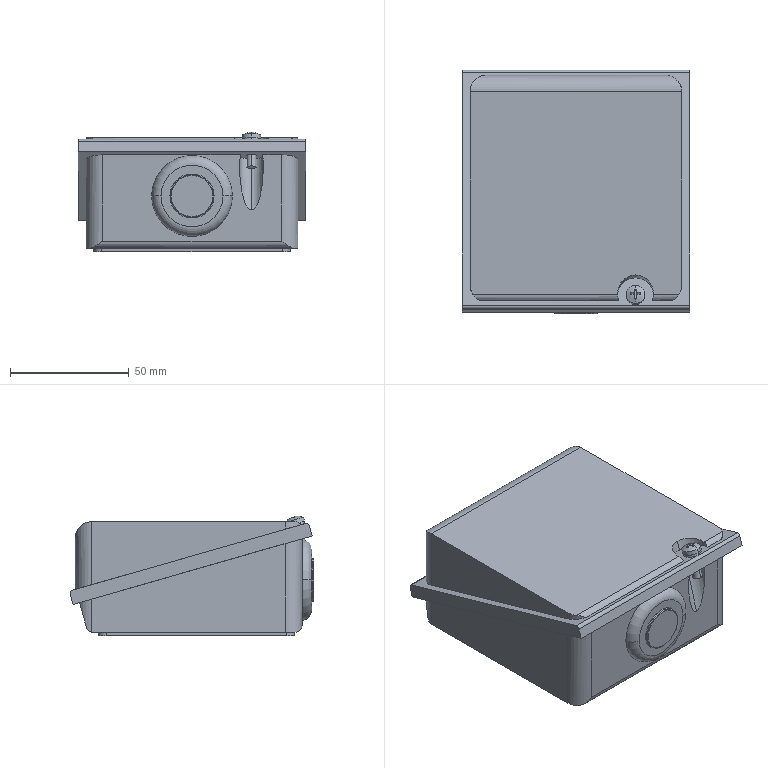Part | STEP file | G3L22N30-MM02TNNTNXH6-Part-8 | 1 solid | 77 faces | box 95.6 x 102.514 x 50.357 mm | volume 408063 mm3 | plane 38 | cylinder 31 | torus 6 | sphere 2 | commonest cylinder face diameters 14 x9 6 x4 6.82 x4 2.6 x2 4 x2 7.6 x2